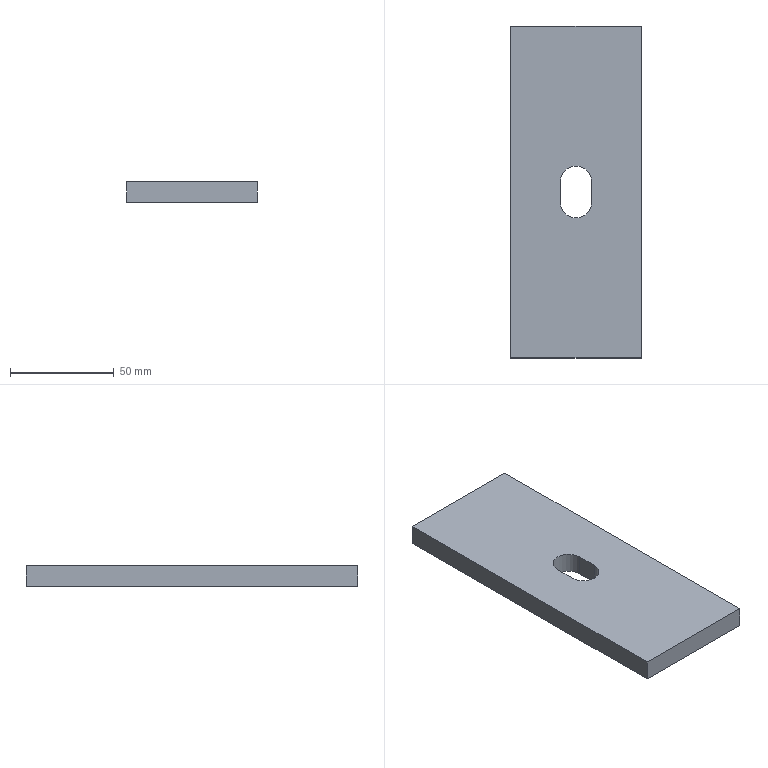Part | STEP file | E3-计量楼梯底Plate 1 | 1 solid | 10 faces | box 63 x 160 x 10 mm | volume 97533 mm3 | plane 8 | cylinder 2 | commonest cylinder face diameters 15 x2
STEP:
#1=CARTESIAN_POINT('',(0.,0.,0.));
#2=DIRECTION('',(0.,0.,1.));
#3=DIRECTION('',(1.,0.,0.));
#4=AXIS2_PLACEMENT_3D('',#1,#2,#3);
#5=CARTESIAN_POINT('',(-31.5,160.,0.));
#6=VERTEX_POINT('',#5);
#7=CARTESIAN_POINT('',(-31.5,0.,0.));
#8=VERTEX_POINT('',#7);
#9=CARTESIAN_POINT('',(-31.5,160.,0.));
#10=DIRECTION('',(0.,-1.,0.));
#11=VECTOR('',#10,1.);
#12=LINE('',#9,#11);
#13=CARTESIAN_POINT('',(0.,0.,0.));
#14=DIRECTION('',(0.,0.,-1.));
#15=DIRECTION('',(1.,0.,0.));
#16=AXIS2_PLACEMENT_3D('',#13,#14,#15);
#17=PLANE('',#16);
#18=CARTESIAN_POINT('',(-31.5,-160.));
#19=DIRECTION('',(0.,1.));
#20=VECTOR('',#19,1.);
#21=LINE('',#18,#20);
#22=(GEOMETRIC_REPRESENTATION_CONTEXT(2)PARAMETRIC_REPRESENTATION_CONTEXT()REPRESENTATION_CONTEXT('',''));
#23=DEFINITIONAL_REPRESENTATION('',(#21),#22);
#24=PCURVE('',#17,#23);
#25=CARTESIAN_POINT('',(-31.5,160.,-10.));
#26=DIRECTION('',(1.,0.,0.));
#27=DIRECTION('',(0.,1.,0.));
#28=AXIS2_PLACEMENT_3D('',#25,#26,#27);
#29=PLANE('',#28);
#30=CARTESIAN_POINT('',(0.,10.));
#31=DIRECTION('',(-1.,0.));
#32=VECTOR('',#31,1.);
#33=LINE('',#30,#32);
#34=(GEOMETRIC_REPRESENTATION_CONTEXT(2)PARAMETRIC_REPRESENTATION_CONTEXT()REPRESENTATION_CONTEXT('',''));
#35=DEFINITIONAL_REPRESENTATION('',(#33),#34);
#36=PCURVE('',#29,#35);
#37=SURFACE_CURVE('',#12,(#24,#36),.PCURVE_S1.);
#38=EDGE_CURVE('',#6,#8,#37,.T.);
#39=ORIENTED_EDGE('',*,*,#38,.T.);
#40=CARTESIAN_POINT('',(31.5,0.,0.));
#41=VERTEX_POINT('',#40);
#42=CARTESIAN_POINT('',(-31.5,0.,0.));
#43=DIRECTION('',(1.,0.,0.));
#44=VECTOR('',#43,1.);
#45=LINE('',#42,#44);
#46=CARTESIAN_POINT('',(-31.5,0.));
#47=DIRECTION('',(1.,0.));
#48=VECTOR('',#47,1.);
#49=LINE('',#46,#48);
#50=(GEOMETRIC_REPRESENTATION_CONTEXT(2)PARAMETRIC_REPRESENTATION_CONTEXT()REPRESENTATION_CONTEXT('',''));
#51=DEFINITIONAL_REPRESENTATION('',(#49),#50);
#52=PCURVE('',#17,#51);
#53=CARTESIAN_POINT('',(-31.5,0.,-10.));
#54=DIRECTION('',(0.,1.,0.));
#55=DIRECTION('',(0.,0.,-1.));
#56=AXIS2_PLACEMENT_3D('',#53,#54,#55);
#57=PLANE('',#56);
#58=CARTESIAN_POINT('',(-10.,0.));
#59=DIRECTION('',(0.,-1.));
#60=VECTOR('',#59,1.);
#61=LINE('',#58,#60);
#62=(GEOMETRIC_REPRESENTATION_CONTEXT(2)PARAMETRIC_REPRESENTATION_CONTEXT()REPRESENTATION_CONTEXT('',''));
#63=DEFINITIONAL_REPRESENTATION('',(#61),#62);
#64=PCURVE('',#57,#63);
#65=SURFACE_CURVE('',#45,(#52,#64),.PCURVE_S1.);
#66=EDGE_CURVE('',#8,#41,#65,.T.);
#67=ORIENTED_EDGE('',*,*,#66,.T.);
#68=CARTESIAN_POINT('',(31.5,160.,0.));
#69=VERTEX_POINT('',#68);
#70=CARTESIAN_POINT('',(31.5,160.,0.));
#71=DIRECTION('',(0.,1.,0.));
#72=VECTOR('',#71,1.);
#73=LINE('',#70,#72);
#74=CARTESIAN_POINT('',(31.5,-160.));
#75=DIRECTION('',(0.,-1.));
#76=VECTOR('',#75,1.);
#77=LINE('',#74,#76);
#78=(GEOMETRIC_REPRESENTATION_CONTEXT(2)PARAMETRIC_REPRESENTATION_CONTEXT()REPRESENTATION_CONTEXT('',''));
#79=DEFINITIONAL_REPRESENTATION('',(#77),#78);
#80=PCURVE('',#17,#79);
#81=CARTESIAN_POINT('',(31.5,160.,-10.));
#82=DIRECTION('',(-1.,0.,0.));
#83=DIRECTION('',(0.,-1.,0.));
#84=AXIS2_PLACEMENT_3D('',#81,#82,#83);
#85=PLANE('',#84);
#86=CARTESIAN_POINT('',(0.,10.));
#87=DIRECTION('',(-1.,0.));
#88=VECTOR('',#87,1.);
#89=LINE('',#86,#88);
#90=(GEOMETRIC_REPRESENTATION_CONTEXT(2)PARAMETRIC_REPRESENTATION_CONTEXT()REPRESENTATION_CONTEXT('',''));
#91=DEFINITIONAL_REPRESENTATION('',(#89),#90);
#92=PCURVE('',#85,#91);
#93=SURFACE_CURVE('',#73,(#80,#92),.PCURVE_S1.);
#94=EDGE_CURVE('',#41,#69,#93,.T.);
#95=ORIENTED_EDGE('',*,*,#94,.T.);
#96=CARTESIAN_POINT('',(-31.5,160.,0.));
#97=DIRECTION('',(-1.,0.,0.));
#98=VECTOR('',#97,1.);
#99=LINE('',#96,#98);
#100=CARTESIAN_POINT('',(-31.5,-160.));
#101=DIRECTION('',(-1.,0.));
#102=VECTOR('',#101,1.);
#103=LINE('',#100,#102);
#104=(GEOMETRIC_REPRESENTATION_CONTEXT(2)PARAMETRIC_REPRESENTATION_CONTEXT()REPRESENTATION_CONTEXT('',''));
#105=DEFINITIONAL_REPRESENTATION('',(#103),#104);
#106=PCURVE('',#17,#105);
#107=CARTESIAN_POINT('',(-31.5,160.,-10.));
#108=DIRECTION('',(0.,-1.,0.));
#109=DIRECTION('',(0.,0.,1.));
#110=AXIS2_PLACEMENT_3D('',#107,#108,#109);
#111=PLANE('',#110);
#112=CARTESIAN_POINT('',(10.,0.));
#113=DIRECTION('',(0.,1.));
#114=VECTOR('',#113,1.);
#115=LINE('',#112,#114);
#116=(GEOMETRIC_REPRESENTATION_CONTEXT(2)PARAMETRIC_REPRESENTATION_CONTEXT()REPRESENTATION_CONTEXT('',''));
#117=DEFINITIONAL_REPRESENTATION('',(#115),#116);
#118=PCURVE('',#111,#117);
#119=SURFACE_CURVE('',#99,(#106,#118),.PCURVE_S1.);
#120=EDGE_CURVE('',#69,#6,#119,.T.);
#121=ORIENTED_EDGE('',*,*,#120,.T.);
#122=EDGE_LOOP('',(#39,#67,#95,#121));
#123=FACE_BOUND('',#122,.T.);
#124=CARTESIAN_POINT('',(-7.5,75.,0.));
#125=VERTEX_POINT('',#124);
#126=CARTESIAN_POINT('',(-7.5,85.,0.));
#127=VERTEX_POINT('',#126);
#128=CARTESIAN_POINT('',(-7.5,75.,0.));
#129=DIRECTION('',(0.,1.,0.));
#130=VECTOR('',#129,1.);
#131=LINE('',#128,#130);
#132=CARTESIAN_POINT('',(-7.5,-75.));
#133=DIRECTION('',(0.,-1.));
#134=VECTOR('',#133,1.);
#135=LINE('',#132,#134);
#136=(GEOMETRIC_REPRESENTATION_CONTEXT(2)PARAMETRIC_REPRESENTATION_CONTEXT()REPRESENTATION_CONTEXT('',''));
#137=DEFINITIONAL_REPRESENTATION('',(#135),#136);
#138=PCURVE('',#17,#137);
#139=CARTESIAN_POINT('',(-7.5,75.,-10.));
#140=DIRECTION('',(-1.,0.,0.));
#141=DIRECTION('',(0.,-1.,0.));
#142=AXIS2_PLACEMENT_3D('',#139,#140,#141);
#143=PLANE('',#142);
#144=CARTESIAN_POINT('',(0.,10.));
#145=DIRECTION('',(-1.,0.));
#146=VECTOR('',#145,1.);
#147=LINE('',#144,#146);
#148=(GEOMETRIC_REPRESENTATION_CONTEXT(2)PARAMETRIC_REPRESENTATION_CONTEXT()REPRESENTATION_CONTEXT('',''));
#149=DEFINITIONAL_REPRESENTATION('',(#147),#148);
#150=PCURVE('',#143,#149);
#151=SURFACE_CURVE('',#131,(#138,#150),.PCURVE_S1.);
#152=EDGE_CURVE('',#125,#127,#151,.T.);
#153=ORIENTED_EDGE('',*,*,#152,.T.);
#154=CARTESIAN_POINT('',(7.5,85.,0.));
#155=VERTEX_POINT('',#154);
#156=CARTESIAN_POINT('',(0.,85.,0.));
#157=DIRECTION('',(0.,0.,1.));
#158=DIRECTION('',(1.,0.,0.));
#159=AXIS2_PLACEMENT_3D('',#156,#157,#158);
#160=CIRCLE('',#159,7.5);
#161=CARTESIAN_POINT('',(7.5,-85.));
#162=CARTESIAN_POINT('',(7.5,-97.99));
#163=CARTESIAN_POINT('',(-3.75,-91.495));
#164=CARTESIAN_POINT('',(-15.,-85.));
#165=CARTESIAN_POINT('',(-3.75,-78.505));
#166=CARTESIAN_POINT('',(7.5,-72.01));
#167=CARTESIAN_POINT('',(7.5,-85.));
#168=(BOUNDED_CURVE()B_SPLINE_CURVE(2,(#161,#162,#163,#164,#165,#166,#167),.UNSPECIFIED.,.T.,.F.)B_SPLINE_CURVE_WITH_KNOTS((1,2,2,2,2,1),(-2.094,0.,2.094,4.189,6.283,8.378),.UNSPECIFIED.)CURVE()GEOMETRIC_REPRESENTATION_ITEM()RATIONAL_B_SPLINE_CURVE((1.,0.5,1.,0.5,1.,0.5,1.))REPRESENTATION_ITEM(''));
#169=(GEOMETRIC_REPRESENTATION_CONTEXT(2)PARAMETRIC_REPRESENTATION_CONTEXT()REPRESENTATION_CONTEXT('',''));
#170=DEFINITIONAL_REPRESENTATION('',(#168),#169);
#171=PCURVE('',#17,#170);
#172=CARTESIAN_POINT('',(0.,85.,-10.));
#173=DIRECTION('',(0.,0.,-1.));
#174=DIRECTION('',(1.,0.,0.));
#175=AXIS2_PLACEMENT_3D('',#172,#173,#174);
#176=CYLINDRICAL_SURFACE('',#175,7.5);
#177=CARTESIAN_POINT('',(6.283,-10.));
#178=DIRECTION('',(-1.,0.));
#179=VECTOR('',#178,1.);
#180=LINE('',#177,#179);
#181=(GEOMETRIC_REPRESENTATION_CONTEXT(2)PARAMETRIC_REPRESENTATION_CONTEXT()REPRESENTATION_CONTEXT('',''));
#182=DEFINITIONAL_REPRESENTATION('',(#180),#181);
#183=PCURVE('',#176,#182);
#184=SURFACE_CURVE('',#160,(#171,#183),.PCURVE_S1.);
#185=EDGE_CURVE('',#155,#127,#184,.T.);
#186=ORIENTED_EDGE('',*,*,#185,.F.);
#187=CARTESIAN_POINT('',(7.5,75.,0.));
#188=VERTEX_POINT('',#187);
#189=CARTESIAN_POINT('',(7.5,75.,0.));
#190=DIRECTION('',(0.,1.,0.));
#191=VECTOR('',#190,1.);
#192=LINE('',#189,#191);
#193=CARTESIAN_POINT('',(7.5,-75.));
#194=DIRECTION('',(0.,-1.));
#195=VECTOR('',#194,1.);
#196=LINE('',#193,#195);
#197=(GEOMETRIC_REPRESENTATION_CONTEXT(2)PARAMETRIC_REPRESENTATION_CONTEXT()REPRESENTATION_CONTEXT('',''));
#198=DEFINITIONAL_REPRESENTATION('',(#196),#197);
#199=PCURVE('',#17,#198);
#200=CARTESIAN_POINT('',(7.5,75.,0.));
#201=DIRECTION('',(1.,0.,0.));
#202=DIRECTION('',(0.,1.,0.));
#203=AXIS2_PLACEMENT_3D('',#200,#201,#202);
#204=PLANE('',#203);
#205=CARTESIAN_POINT('',(0.,0.));
#206=DIRECTION('',(1.,0.));
#207=VECTOR('',#206,1.);
#208=LINE('',#205,#207);
#209=(GEOMETRIC_REPRESENTATION_CONTEXT(2)PARAMETRIC_REPRESENTATION_CONTEXT()REPRESENTATION_CONTEXT('',''));
#210=DEFINITIONAL_REPRESENTATION('',(#208),#209);
#211=PCURVE('',#204,#210);
#212=SURFACE_CURVE('',#192,(#199,#211),.PCURVE_S1.);
#213=EDGE_CURVE('',#188,#155,#212,.T.);
#214=ORIENTED_EDGE('',*,*,#213,.F.);
#215=CARTESIAN_POINT('',(0.,75.,0.));
#216=DIRECTION('',(0.,0.,1.));
#217=DIRECTION('',(1.,0.,0.));
#218=AXIS2_PLACEMENT_3D('',#215,#216,#217);
#219=CIRCLE('',#218,7.5);
#220=CARTESIAN_POINT('',(7.5,-75.));
#221=CARTESIAN_POINT('',(7.5,-87.99));
#222=CARTESIAN_POINT('',(-3.75,-81.495));
#223=CARTESIAN_POINT('',(-15.,-75.));
#224=CARTESIAN_POINT('',(-3.75,-68.505));
#225=CARTESIAN_POINT('',(7.5,-62.01));
#226=CARTESIAN_POINT('',(7.5,-75.));
#227=(BOUNDED_CURVE()B_SPLINE_CURVE(2,(#220,#221,#222,#223,#224,#225,#226),.UNSPECIFIED.,.T.,.F.)B_SPLINE_CURVE_WITH_KNOTS((1,2,2,2,2,1),(-2.094,0.,2.094,4.189,6.283,8.378),.UNSPECIFIED.)CURVE()GEOMETRIC_REPRESENTATION_ITEM()RATIONAL_B_SPLINE_CURVE((1.,0.5,1.,0.5,1.,0.5,1.))REPRESENTATION_ITEM(''));
#228=(GEOMETRIC_REPRESENTATION_CONTEXT(2)PARAMETRIC_REPRESENTATION_CONTEXT()REPRESENTATION_CONTEXT('',''));
#229=DEFINITIONAL_REPRESENTATION('',(#227),#228);
#230=PCURVE('',#17,#229);
#231=CARTESIAN_POINT('',(0.,75.,-10.));
#232=DIRECTION('',(0.,0.,-1.));
#233=DIRECTION('',(1.,0.,0.));
#234=AXIS2_PLACEMENT_3D('',#231,#232,#233);
#235=CYLINDRICAL_SURFACE('',#234,7.5);
#236=CARTESIAN_POINT('',(6.283,-10.));
#237=DIRECTION('',(-1.,0.));
#238=VECTOR('',#237,1.);
#239=LINE('',#236,#238);
#240=(GEOMETRIC_REPRESENTATION_CONTEXT(2)PARAMETRIC_REPRESENTATION_CONTEXT()REPRESENTATION_CONTEXT('',''));
#241=DEFINITIONAL_REPRESENTATION('',(#239),#240);
#242=PCURVE('',#235,#241);
#243=SURFACE_CURVE('',#219,(#230,#242),.PCURVE_S1.);
#244=EDGE_CURVE('',#125,#188,#243,.T.);
#245=ORIENTED_EDGE('',*,*,#244,.F.);
#246=EDGE_LOOP('',(#153,#186,#214,#245));
#247=FACE_BOUND('',#246,.T.);
#248=ADVANCED_FACE('',(#123,#247),#17,.F.);
#249=ORIENTED_EDGE('',*,*,#38,.F.);
#250=CARTESIAN_POINT('',(-31.5,160.,-10.));
#251=VERTEX_POINT('',#250);
#252=CARTESIAN_POINT('',(-31.5,160.,-10.));
#253=DIRECTION('',(0.,0.,1.));
#254=VECTOR('',#253,1.);
#255=LINE('',#252,#254);
#256=CARTESIAN_POINT('',(0.,0.));
#257=DIRECTION('',(0.,1.));
#258=VECTOR('',#257,1.);
#259=LINE('',#256,#258);
#260=(GEOMETRIC_REPRESENTATION_CONTEXT(2)PARAMETRIC_REPRESENTATION_CONTEXT()REPRESENTATION_CONTEXT('',''));
#261=DEFINITIONAL_REPRESENTATION('',(#259),#260);
#262=PCURVE('',#29,#261);
#263=CARTESIAN_POINT('',(0.,0.));
#264=DIRECTION('',(1.,0.));
#265=VECTOR('',#264,1.);
#266=LINE('',#263,#265);
#267=(GEOMETRIC_REPRESENTATION_CONTEXT(2)PARAMETRIC_REPRESENTATION_CONTEXT()REPRESENTATION_CONTEXT('',''));
#268=DEFINITIONAL_REPRESENTATION('',(#266),#267);
#269=PCURVE('',#111,#268);
#270=SURFACE_CURVE('',#255,(#262,#269),.PCURVE_S1.);
#271=EDGE_CURVE('',#251,#6,#270,.T.);
#272=ORIENTED_EDGE('',*,*,#271,.F.);
#273=CARTESIAN_POINT('',(-31.5,0.,-10.));
#274=VERTEX_POINT('',#273);
#275=CARTESIAN_POINT('',(-31.5,160.,-10.));
#276=DIRECTION('',(0.,-1.,0.));
#277=VECTOR('',#276,1.);
#278=LINE('',#275,#277);
#279=CARTESIAN_POINT('',(0.,0.));
#280=DIRECTION('',(-1.,0.));
#281=VECTOR('',#280,1.);
#282=LINE('',#279,#281);
#283=(GEOMETRIC_REPRESENTATION_CONTEXT(2)PARAMETRIC_REPRESENTATION_CONTEXT()REPRESENTATION_CONTEXT('',''));
#284=DEFINITIONAL_REPRESENTATION('',(#282),#283);
#285=PCURVE('',#29,#284);
#286=CARTESIAN_POINT('',(0.,0.,-10.));
#287=DIRECTION('',(0.,0.,-1.));
#288=DIRECTION('',(1.,0.,0.));
#289=AXIS2_PLACEMENT_3D('',#286,#287,#288);
#290=PLANE('',#289);
#291=CARTESIAN_POINT('',(-31.5,-160.));
#292=DIRECTION('',(0.,1.));
#293=VECTOR('',#292,1.);
#294=LINE('',#291,#293);
#295=(GEOMETRIC_REPRESENTATION_CONTEXT(2)PARAMETRIC_REPRESENTATION_CONTEXT()REPRESENTATION_CONTEXT('',''));
#296=DEFINITIONAL_REPRESENTATION('',(#294),#295);
#297=PCURVE('',#290,#296);
#298=SURFACE_CURVE('',#278,(#285,#297),.PCURVE_S1.);
#299=EDGE_CURVE('',#251,#274,#298,.T.);
#300=ORIENTED_EDGE('',*,*,#299,.T.);
#301=CARTESIAN_POINT('',(-31.5,0.,-10.));
#302=DIRECTION('',(0.,0.,1.));
#303=VECTOR('',#302,1.);
#304=LINE('',#301,#303);
#305=CARTESIAN_POINT('',(-160.,0.));
#306=DIRECTION('',(0.,1.));
#307=VECTOR('',#306,1.);
#308=LINE('',#305,#307);
#309=(GEOMETRIC_REPRESENTATION_CONTEXT(2)PARAMETRIC_REPRESENTATION_CONTEXT()REPRESENTATION_CONTEXT('',''));
#310=DEFINITIONAL_REPRESENTATION('',(#308),#309);
#311=PCURVE('',#29,#310);
#312=CARTESIAN_POINT('',(0.,0.));
#313=DIRECTION('',(-1.,0.));
#314=VECTOR('',#313,1.);
#315=LINE('',#312,#314);
#316=(GEOMETRIC_REPRESENTATION_CONTEXT(2)PARAMETRIC_REPRESENTATION_CONTEXT()REPRESENTATION_CONTEXT('',''));
#317=DEFINITIONAL_REPRESENTATION('',(#315),#316);
#318=PCURVE('',#57,#317);
#319=SURFACE_CURVE('',#304,(#311,#318),.PCURVE_S1.);
#320=EDGE_CURVE('',#274,#8,#319,.T.);
#321=ORIENTED_EDGE('',*,*,#320,.T.);
#322=EDGE_LOOP('',(#249,#272,#300,#321));
#323=FACE_BOUND('',#322,.T.);
#324=ADVANCED_FACE('',(#323),#29,.F.);
#325=ORIENTED_EDGE('',*,*,#66,.F.);
#326=ORIENTED_EDGE('',*,*,#320,.F.);
#327=CARTESIAN_POINT('',(31.5,0.,-10.));
#328=VERTEX_POINT('',#327);
#329=CARTESIAN_POINT('',(-31.5,0.,-10.));
#330=DIRECTION('',(1.,0.,0.));
#331=VECTOR('',#330,1.);
#332=LINE('',#329,#331);
#333=CARTESIAN_POINT('',(0.,0.));
#334=DIRECTION('',(0.,-1.));
#335=VECTOR('',#334,1.);
#336=LINE('',#333,#335);
#337=(GEOMETRIC_REPRESENTATION_CONTEXT(2)PARAMETRIC_REPRESENTATION_CONTEXT()REPRESENTATION_CONTEXT('',''));
#338=DEFINITIONAL_REPRESENTATION('',(#336),#337);
#339=PCURVE('',#57,#338);
#340=CARTESIAN_POINT('',(-31.5,0.));
#341=DIRECTION('',(1.,0.));
#342=VECTOR('',#341,1.);
#343=LINE('',#340,#342);
#344=(GEOMETRIC_REPRESENTATION_CONTEXT(2)PARAMETRIC_REPRESENTATION_CONTEXT()REPRESENTATION_CONTEXT('',''));
#345=DEFINITIONAL_REPRESENTATION('',(#343),#344);
#346=PCURVE('',#290,#345);
#347=SURFACE_CURVE('',#332,(#339,#346),.PCURVE_S1.);
#348=EDGE_CURVE('',#274,#328,#347,.T.);
#349=ORIENTED_EDGE('',*,*,#348,.T.);
#350=CARTESIAN_POINT('',(31.5,0.,-10.));
#351=DIRECTION('',(0.,0.,1.));
#352=VECTOR('',#351,1.);
#353=LINE('',#350,#352);
#354=CARTESIAN_POINT('',(0.,-63.));
#355=DIRECTION('',(-1.,0.));
#356=VECTOR('',#355,1.);
#357=LINE('',#354,#356);
#358=(GEOMETRIC_REPRESENTATION_CONTEXT(2)PARAMETRIC_REPRESENTATION_CONTEXT()REPRESENTATION_CONTEXT('',''));
#359=DEFINITIONAL_REPRESENTATION('',(#357),#358);
#360=PCURVE('',#57,#359);
#361=CARTESIAN_POINT('',(160.,0.));
#362=DIRECTION('',(0.,1.));
#363=VECTOR('',#362,1.);
#364=LINE('',#361,#363);
#365=(GEOMETRIC_REPRESENTATION_CONTEXT(2)PARAMETRIC_REPRESENTATION_CONTEXT()REPRESENTATION_CONTEXT('',''));
#366=DEFINITIONAL_REPRESENTATION('',(#364),#365);
#367=PCURVE('',#85,#366);
#368=SURFACE_CURVE('',#353,(#360,#367),.PCURVE_S1.);
#369=EDGE_CURVE('',#328,#41,#368,.T.);
#370=ORIENTED_EDGE('',*,*,#369,.T.);
#371=EDGE_LOOP('',(#325,#326,#349,#370));
#372=FACE_BOUND('',#371,.T.);
#373=ADVANCED_FACE('',(#372),#57,.F.);
#374=ORIENTED_EDGE('',*,*,#94,.F.);
#375=ORIENTED_EDGE('',*,*,#369,.F.);
#376=CARTESIAN_POINT('',(31.5,160.,-10.));
#377=VERTEX_POINT('',#376);
#378=CARTESIAN_POINT('',(31.5,160.,-10.));
#379=DIRECTION('',(0.,1.,0.));
#380=VECTOR('',#379,1.);
#381=LINE('',#378,#380);
#382=CARTESIAN_POINT('',(0.,0.));
#383=DIRECTION('',(-1.,0.));
#384=VECTOR('',#383,1.);
#385=LINE('',#382,#384);
#386=(GEOMETRIC_REPRESENTATION_CONTEXT(2)PARAMETRIC_REPRESENTATION_CONTEXT()REPRESENTATION_CONTEXT('',''));
#387=DEFINITIONAL_REPRESENTATION('',(#385),#386);
#388=PCURVE('',#85,#387);
#389=CARTESIAN_POINT('',(31.5,-160.));
#390=DIRECTION('',(0.,-1.));
#391=VECTOR('',#390,1.);
#392=LINE('',#389,#391);
#393=(GEOMETRIC_REPRESENTATION_CONTEXT(2)PARAMETRIC_REPRESENTATION_CONTEXT()REPRESENTATION_CONTEXT('',''));
#394=DEFINITIONAL_REPRESENTATION('',(#392),#393);
#395=PCURVE('',#290,#394);
#396=SURFACE_CURVE('',#381,(#388,#395),.PCURVE_S1.);
#397=EDGE_CURVE('',#328,#377,#396,.T.);
#398=ORIENTED_EDGE('',*,*,#397,.T.);
#399=CARTESIAN_POINT('',(31.5,160.,-10.));
#400=DIRECTION('',(0.,0.,1.));
#401=VECTOR('',#400,1.);
#402=LINE('',#399,#401);
#403=CARTESIAN_POINT('',(0.,0.));
#404=DIRECTION('',(0.,1.));
#405=VECTOR('',#404,1.);
#406=LINE('',#403,#405);
#407=(GEOMETRIC_REPRESENTATION_CONTEXT(2)PARAMETRIC_REPRESENTATION_CONTEXT()REPRESENTATION_CONTEXT('',''));
#408=DEFINITIONAL_REPRESENTATION('',(#406),#407);
#409=PCURVE('',#85,#408);
#410=CARTESIAN_POINT('',(0.,-63.));
#411=DIRECTION('',(1.,0.));
#412=VECTOR('',#411,1.);
#413=LINE('',#410,#412);
#414=(GEOMETRIC_REPRESENTATION_CONTEXT(2)PARAMETRIC_REPRESENTATION_CONTEXT()REPRESENTATION_CONTEXT('',''));
#415=DEFINITIONAL_REPRESENTATION('',(#413),#414);
#416=PCURVE('',#111,#415);
#417=SURFACE_CURVE('',#402,(#409,#416),.PCURVE_S1.);
#418=EDGE_CURVE('',#377,#69,#417,.T.);
#419=ORIENTED_EDGE('',*,*,#418,.T.);
#420=EDGE_LOOP('',(#374,#375,#398,#419));
#421=FACE_BOUND('',#420,.T.);
#422=ADVANCED_FACE('',(#421),#85,.F.);
#423=ORIENTED_EDGE('',*,*,#120,.F.);
#424=ORIENTED_EDGE('',*,*,#418,.F.);
#425=CARTESIAN_POINT('',(-31.5,160.,-10.));
#426=DIRECTION('',(-1.,0.,0.));
#427=VECTOR('',#426,1.);
#428=LINE('',#425,#427);
#429=CARTESIAN_POINT('',(0.,0.));
#430=DIRECTION('',(0.,1.));
#431=VECTOR('',#430,1.);
#432=LINE('',#429,#431);
#433=(GEOMETRIC_REPRESENTATION_CONTEXT(2)PARAMETRIC_REPRESENTATION_CONTEXT()REPRESENTATION_CONTEXT('',''));
#434=DEFINITIONAL_REPRESENTATION('',(#432),#433);
#435=PCURVE('',#111,#434);
#436=CARTESIAN_POINT('',(-31.5,-160.));
#437=DIRECTION('',(-1.,0.));
#438=VECTOR('',#437,1.);
#439=LINE('',#436,#438);
#440=(GEOMETRIC_REPRESENTATION_CONTEXT(2)PARAMETRIC_REPRESENTATION_CONTEXT()REPRESENTATION_CONTEXT('',''));
#441=DEFINITIONAL_REPRESENTATION('',(#439),#440);
#442=PCURVE('',#290,#441);
#443=SURFACE_CURVE('',#428,(#435,#442),.PCURVE_S1.);
#444=EDGE_CURVE('',#377,#251,#443,.T.);
#445=ORIENTED_EDGE('',*,*,#444,.T.);
#446=ORIENTED_EDGE('',*,*,#271,.T.);
#447=EDGE_LOOP('',(#423,#424,#445,#446));
#448=FACE_BOUND('',#447,.T.);
#449=ADVANCED_FACE('',(#448),#111,.F.);
#450=CARTESIAN_POINT('',(7.5,85.,-10.));
#451=VERTEX_POINT('',#450);
#452=CARTESIAN_POINT('',(-7.5,85.,-10.));
#453=VERTEX_POINT('',#452);
#454=CARTESIAN_POINT('',(0.,85.,-10.));
#455=DIRECTION('',(0.,0.,1.));
#456=DIRECTION('',(1.,0.,0.));
#457=AXIS2_PLACEMENT_3D('',#454,#455,#456);
#458=CIRCLE('',#457,7.5);
#459=CARTESIAN_POINT('',(7.5,-85.));
#460=CARTESIAN_POINT('',(7.5,-97.99));
#461=CARTESIAN_POINT('',(-3.75,-91.495));
#462=CARTESIAN_POINT('',(-15.,-85.));
#463=CARTESIAN_POINT('',(-3.75,-78.505));
#464=CARTESIAN_POINT('',(7.5,-72.01));
#465=CARTESIAN_POINT('',(7.5,-85.));
#466=(BOUNDED_CURVE()B_SPLINE_CURVE(2,(#459,#460,#461,#462,#463,#464,#465),.UNSPECIFIED.,.T.,.F.)B_SPLINE_CURVE_WITH_KNOTS((1,2,2,2,2,1),(-2.094,0.,2.094,4.189,6.283,8.378),.UNSPECIFIED.)CURVE()GEOMETRIC_REPRESENTATION_ITEM()RATIONAL_B_SPLINE_CURVE((1.,0.5,1.,0.5,1.,0.5,1.))REPRESENTATION_ITEM(''));
#467=(GEOMETRIC_REPRESENTATION_CONTEXT(2)PARAMETRIC_REPRESENTATION_CONTEXT()REPRESENTATION_CONTEXT('',''));
#468=DEFINITIONAL_REPRESENTATION('',(#466),#467);
#469=PCURVE('',#290,#468);
#470=CARTESIAN_POINT('',(6.283,0.));
#471=DIRECTION('',(-1.,0.));
#472=VECTOR('',#471,1.);
#473=LINE('',#470,#472);
#474=(GEOMETRIC_REPRESENTATION_CONTEXT(2)PARAMETRIC_REPRESENTATION_CONTEXT()REPRESENTATION_CONTEXT('',''));
#475=DEFINITIONAL_REPRESENTATION('',(#473),#474);
#476=PCURVE('',#176,#475);
#477=SURFACE_CURVE('',#458,(#469,#476),.PCURVE_S1.);
#478=EDGE_CURVE('',#451,#453,#477,.T.);
#479=ORIENTED_EDGE('',*,*,#478,.T.);
#480=CARTESIAN_POINT('',(-7.5,75.,-10.));
#481=VERTEX_POINT('',#480);
#482=CARTESIAN_POINT('',(-7.5,75.,-10.));
#483=DIRECTION('',(0.,1.,0.));
#484=VECTOR('',#483,1.);
#485=LINE('',#482,#484);
#486=CARTESIAN_POINT('',(-7.5,-75.));
#487=DIRECTION('',(0.,-1.));
#488=VECTOR('',#487,1.);
#489=LINE('',#486,#488);
#490=(GEOMETRIC_REPRESENTATION_CONTEXT(2)PARAMETRIC_REPRESENTATION_CONTEXT()REPRESENTATION_CONTEXT('',''));
#491=DEFINITIONAL_REPRESENTATION('',(#489),#490);
#492=PCURVE('',#290,#491);
#493=CARTESIAN_POINT('',(0.,0.));
#494=DIRECTION('',(-1.,0.));
#495=VECTOR('',#494,1.);
#496=LINE('',#493,#495);
#497=(GEOMETRIC_REPRESENTATION_CONTEXT(2)PARAMETRIC_REPRESENTATION_CONTEXT()REPRESENTATION_CONTEXT('',''));
#498=DEFINITIONAL_REPRESENTATION('',(#496),#497);
#499=PCURVE('',#143,#498);
#500=SURFACE_CURVE('',#485,(#492,#499),.PCURVE_S1.);
#501=EDGE_CURVE('',#481,#453,#500,.T.);
#502=ORIENTED_EDGE('',*,*,#501,.F.);
#503=CARTESIAN_POINT('',(7.5,75.,-10.));
#504=VERTEX_POINT('',#503);
#505=CARTESIAN_POINT('',(0.,75.,-10.));
#506=DIRECTION('',(0.,0.,1.));
#507=DIRECTION('',(1.,0.,0.));
#508=AXIS2_PLACEMENT_3D('',#505,#506,#507);
#509=CIRCLE('',#508,7.5);
#510=CARTESIAN_POINT('',(7.5,-75.));
#511=CARTESIAN_POINT('',(7.5,-87.99));
#512=CARTESIAN_POINT('',(-3.75,-81.495));
#513=CARTESIAN_POINT('',(-15.,-75.));
#514=CARTESIAN_POINT('',(-3.75,-68.505));
#515=CARTESIAN_POINT('',(7.5,-62.01));
#516=CARTESIAN_POINT('',(7.5,-75.));
#517=(BOUNDED_CURVE()B_SPLINE_CURVE(2,(#510,#511,#512,#513,#514,#515,#516),.UNSPECIFIED.,.T.,.F.)B_SPLINE_CURVE_WITH_KNOTS((1,2,2,2,2,1),(-2.094,0.,2.094,4.189,6.283,8.378),.UNSPECIFIED.)CURVE()GEOMETRIC_REPRESENTATION_ITEM()RATIONAL_B_SPLINE_CURVE((1.,0.5,1.,0.5,1.,0.5,1.))REPRESENTATION_ITEM(''));
#518=(GEOMETRIC_REPRESENTATION_CONTEXT(2)PARAMETRIC_REPRESENTATION_CONTEXT()REPRESENTATION_CONTEXT('',''));
#519=DEFINITIONAL_REPRESENTATION('',(#517),#518);
#520=PCURVE('',#290,#519);
#521=CARTESIAN_POINT('',(6.283,0.));
#522=DIRECTION('',(-1.,0.));
#523=VECTOR('',#522,1.);
#524=LINE('',#521,#523);
#525=(GEOMETRIC_REPRESENTATION_CONTEXT(2)PARAMETRIC_REPRESENTATION_CONTEXT()REPRESENTATION_CONTEXT('',''));
#526=DEFINITIONAL_REPRESENTATION('',(#524),#525);
#527=PCURVE('',#235,#526);
#528=SURFACE_CURVE('',#509,(#520,#527),.PCURVE_S1.);
#529=EDGE_CURVE('',#481,#504,#528,.T.);
#530=ORIENTED_EDGE('',*,*,#529,.T.);
#531=CARTESIAN_POINT('',(7.5,75.,-10.));
#532=DIRECTION('',(0.,1.,0.));
#533=VECTOR('',#532,1.);
#534=LINE('',#531,#533);
#535=CARTESIAN_POINT('',(7.5,-75.));
#536=DIRECTION('',(0.,-1.));
#537=VECTOR('',#536,1.);
#538=LINE('',#535,#537);
#539=(GEOMETRIC_REPRESENTATION_CONTEXT(2)PARAMETRIC_REPRESENTATION_CONTEXT()REPRESENTATION_CONTEXT('',''));
#540=DEFINITIONAL_REPRESENTATION('',(#538),#539);
#541=PCURVE('',#290,#540);
#542=CARTESIAN_POINT('',(0.,-10.));
#543=DIRECTION('',(1.,0.));
#544=VECTOR('',#543,1.);
#545=LINE('',#542,#544);
#546=(GEOMETRIC_REPRESENTATION_CONTEXT(2)PARAMETRIC_REPRESENTATION_CONTEXT()REPRESENTATION_CONTEXT('',''));
#547=DEFINITIONAL_REPRESENTATION('',(#545),#546);
#548=PCURVE('',#204,#547);
#549=SURFACE_CURVE('',#534,(#541,#548),.PCURVE_S1.);
#550=EDGE_CURVE('',#504,#451,#549,.T.);
#551=ORIENTED_EDGE('',*,*,#550,.T.);
#552=EDGE_LOOP('',(#479,#502,#530,#551));
#553=FACE_BOUND('',#552,.T.);
#554=ORIENTED_EDGE('',*,*,#299,.F.);
#555=ORIENTED_EDGE('',*,*,#444,.F.);
#556=ORIENTED_EDGE('',*,*,#397,.F.);
#557=ORIENTED_EDGE('',*,*,#348,.F.);
#558=EDGE_LOOP('',(#554,#555,#556,#557));
#559=FACE_BOUND('',#558,.T.);
#560=ADVANCED_FACE('',(#553,#559),#290,.T.);
#561=CARTESIAN_POINT('',(7.5,85.,0.));
#562=DIRECTION('',(0.,0.,1.));
#563=VECTOR('',#562,1.);
#564=LINE('',#561,#563);
#565=CARTESIAN_POINT('',(6.283,-10.));
#566=DIRECTION('',(0.,-1.));
#567=VECTOR('',#566,1.);
#568=LINE('',#565,#567);
#569=(GEOMETRIC_REPRESENTATION_CONTEXT(2)PARAMETRIC_REPRESENTATION_CONTEXT()REPRESENTATION_CONTEXT('',''));
#570=DEFINITIONAL_REPRESENTATION('',(#568),#569);
#571=PCURVE('',#176,#570);
#572=CARTESIAN_POINT('',(10.,0.));
#573=DIRECTION('',(0.,1.));
#574=VECTOR('',#573,1.);
#575=LINE('',#572,#574);
#576=(GEOMETRIC_REPRESENTATION_CONTEXT(2)PARAMETRIC_REPRESENTATION_CONTEXT()REPRESENTATION_CONTEXT('',''));
#577=DEFINITIONAL_REPRESENTATION('',(#575),#576);
#578=PCURVE('',#204,#577);
#579=SURFACE_CURVE('',#564,(#571,#578),.PCURVE_S1.);
#580=EDGE_CURVE('',#451,#155,#579,.T.);
#581=ORIENTED_EDGE('',*,*,#580,.F.);
#582=ORIENTED_EDGE('',*,*,#478,.T.);
#583=CARTESIAN_POINT('',(-7.5,85.,-10.));
#584=DIRECTION('',(0.,0.,-1.));
#585=VECTOR('',#584,1.);
#586=LINE('',#583,#585);
#587=CARTESIAN_POINT('',(3.142,0.));
#588=DIRECTION('',(0.,1.));
#589=VECTOR('',#588,1.);
#590=LINE('',#587,#589);
#591=(GEOMETRIC_REPRESENTATION_CONTEXT(2)PARAMETRIC_REPRESENTATION_CONTEXT()REPRESENTATION_CONTEXT('',''));
#592=DEFINITIONAL_REPRESENTATION('',(#590),#591);
#593=PCURVE('',#176,#592);
#594=CARTESIAN_POINT('',(-10.,0.));
#595=DIRECTION('',(0.,-1.));
#596=VECTOR('',#595,1.);
#597=LINE('',#594,#596);
#598=(GEOMETRIC_REPRESENTATION_CONTEXT(2)PARAMETRIC_REPRESENTATION_CONTEXT()REPRESENTATION_CONTEXT('',''));
#599=DEFINITIONAL_REPRESENTATION('',(#597),#598);
#600=PCURVE('',#143,#599);
#601=SURFACE_CURVE('',#586,(#593,#600),.PCURVE_S1.);
#602=EDGE_CURVE('',#127,#453,#601,.T.);
#603=ORIENTED_EDGE('',*,*,#602,.F.);
#604=ORIENTED_EDGE('',*,*,#185,.F.);
#605=EDGE_LOOP('',(#581,#582,#603,#604));
#606=FACE_BOUND('',#605,.F.);
#607=ADVANCED_FACE('',(#606),#176,.F.);
#608=CARTESIAN_POINT('',(7.5,75.,0.));
#609=DIRECTION('',(0.,0.,1.));
#610=VECTOR('',#609,1.);
#611=LINE('',#608,#610);
#612=CARTESIAN_POINT('',(0.,-10.));
#613=DIRECTION('',(0.,-1.));
#614=VECTOR('',#613,1.);
#615=LINE('',#612,#614);
#616=(GEOMETRIC_REPRESENTATION_CONTEXT(2)PARAMETRIC_REPRESENTATION_CONTEXT()REPRESENTATION_CONTEXT('',''));
#617=DEFINITIONAL_REPRESENTATION('',(#615),#616);
#618=PCURVE('',#235,#617);
#619=CARTESIAN_POINT('',(0.,0.));
#620=DIRECTION('',(0.,1.));
#621=VECTOR('',#620,1.);
#622=LINE('',#619,#621);
#623=(GEOMETRIC_REPRESENTATION_CONTEXT(2)PARAMETRIC_REPRESENTATION_CONTEXT()REPRESENTATION_CONTEXT('',''));
#624=DEFINITIONAL_REPRESENTATION('',(#622),#623);
#625=PCURVE('',#204,#624);
#626=SURFACE_CURVE('',#611,(#618,#625),.PCURVE_S1.);
#627=EDGE_CURVE('',#504,#188,#626,.T.);
#628=ORIENTED_EDGE('',*,*,#627,.T.);
#629=ORIENTED_EDGE('',*,*,#244,.F.);
#630=CARTESIAN_POINT('',(-7.5,75.,-10.));
#631=DIRECTION('',(0.,0.,1.));
#632=VECTOR('',#631,1.);
#633=LINE('',#630,#632);
#634=CARTESIAN_POINT('',(3.142,0.));
#635=DIRECTION('',(0.,-1.));
#636=VECTOR('',#635,1.);
#637=LINE('',#634,#636);
#638=(GEOMETRIC_REPRESENTATION_CONTEXT(2)PARAMETRIC_REPRESENTATION_CONTEXT()REPRESENTATION_CONTEXT('',''));
#639=DEFINITIONAL_REPRESENTATION('',(#637),#638);
#640=PCURVE('',#235,#639);
#641=CARTESIAN_POINT('',(0.,0.));
#642=DIRECTION('',(0.,1.));
#643=VECTOR('',#642,1.);
#644=LINE('',#641,#643);
#645=(GEOMETRIC_REPRESENTATION_CONTEXT(2)PARAMETRIC_REPRESENTATION_CONTEXT()REPRESENTATION_CONTEXT('',''));
#646=DEFINITIONAL_REPRESENTATION('',(#644),#645);
#647=PCURVE('',#143,#646);
#648=SURFACE_CURVE('',#633,(#640,#647),.PCURVE_S1.);
#649=EDGE_CURVE('',#481,#125,#648,.T.);
#650=ORIENTED_EDGE('',*,*,#649,.F.);
#651=ORIENTED_EDGE('',*,*,#529,.T.);
#652=EDGE_LOOP('',(#628,#629,#650,#651));
#653=FACE_BOUND('',#652,.F.);
#654=ADVANCED_FACE('',(#653),#235,.F.);
#655=ORIENTED_EDGE('',*,*,#602,.F.);
#656=ORIENTED_EDGE('',*,*,#152,.F.);
#657=ORIENTED_EDGE('',*,*,#649,.F.);
#658=ORIENTED_EDGE('',*,*,#501,.T.);
#659=EDGE_LOOP('',(#655,#656,#657,#658));
#660=FACE_BOUND('',#659,.T.);
#661=ADVANCED_FACE('',(#660),#143,.F.);
#662=ORIENTED_EDGE('',*,*,#580,.F.);
#663=ORIENTED_EDGE('',*,*,#550,.F.);
#664=ORIENTED_EDGE('',*,*,#627,.T.);
#665=ORIENTED_EDGE('',*,*,#213,.T.);
#666=EDGE_LOOP('',(#662,#663,#664,#665));
#667=FACE_BOUND('',#666,.T.);
#668=ADVANCED_FACE('',(#667),#204,.F.);
#669=CLOSED_SHELL('',(#248,#324,#373,#422,#449,#560,#607,#654,#661,#668));
#670=MANIFOLD_SOLID_BREP('',#669);
#671=(LENGTH_UNIT()NAMED_UNIT(*)SI_UNIT(.MILLI.,.METRE.));
#672=UNCERTAINTY_MEASURE_WITH_UNIT(LENGTH_MEASURE(0.0000001),#671,'','');
#673=(NAMED_UNIT(*)PLANE_ANGLE_UNIT()SI_UNIT($,.RADIAN.));
#674=(NAMED_UNIT(*)SI_UNIT($,.STERADIAN.)SOLID_ANGLE_UNIT());
#675=(GEOMETRIC_REPRESENTATION_CONTEXT(3)GLOBAL_UNCERTAINTY_ASSIGNED_CONTEXT((#672))GLOBAL_UNIT_ASSIGNED_CONTEXT((#671,#673,#674))REPRESENTATION_CONTEXT('',''));
#676=ADVANCED_BREP_SHAPE_REPRESENTATION('',(#4,#670),#675);